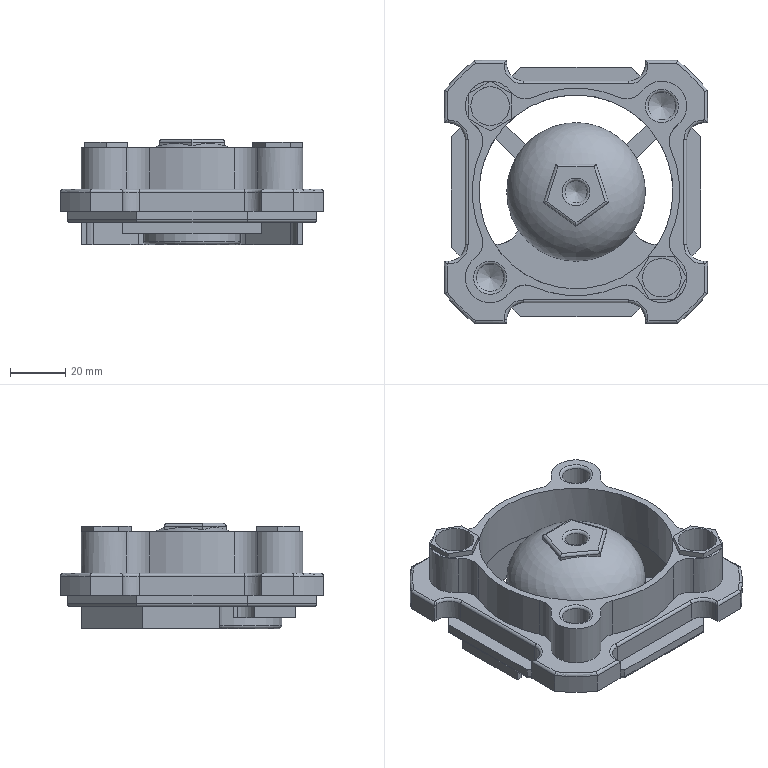NC program | NX | posted with a generic post | part box 95 x 95 x 38 mm
Lines 1358 to 2302 of 59038:
(PLANAR_MILL , TOOL : D20)
N2702 M6
N2704 G54
N2706 G17 G0 G90 X-51.14 Y-59.625 S3000 M3
N2708 G43 Z10. H0
N2710 Z-3.589
N2712 G94 G1 Z-3.789 F2500.
N2714 X-44.435 Y-52.92
N2716 G3 X-44.435 Y-44.435 R6.
N2718 G2 X-44.218 Y-17.351 R19.
N2720 X-44.218 Y17.351 R47.5
N2722 X-17.351 Y44.218 R-19.
N2724 X17.351 Y44.218 R47.5
N2726 X44.218 Y17.351 R-19.
N2728 X44.218 Y-17.351 R47.5
N2730 X17.351 Y-44.218 R-19.
N2732 X-17.351 Y-44.218 R47.5
N2734 X-44.435 Y-44.435 R19.
N2736 G3 X-52.92 Y-44.435 R6.
N2738 G1 X-59.625 Y-51.14
N2740 Z-3.589
N2742 G0 X-51.14 Y-59.625 Z-4.379
N2744 G1 Z-4.579
N2746 X-44.435 Y-52.92
N2748 G3 X-44.435 Y-44.435 R6.
N2750 G2 X-44.218 Y-17.351 R19.
N2752 X-44.218 Y17.351 R47.5
N2754 X-17.351 Y44.218 R-19.
N2756 X17.351 Y44.218 R47.5
N2758 X44.218 Y17.351 R-19.
N2760 X44.218 Y-17.351 R47.5
N2762 X17.351 Y-44.218 R-19.
N2764 X-17.351 Y-44.218 R47.5
N2766 X-44.435 Y-44.435 R19.
N2768 G3 X-52.92 Y-44.435 R6.
N2770 G1 X-59.625 Y-51.14
N2772 Z-4.379
N2774 G0 X-51.14 Y-59.625 Z-5.168
N2776 G1 Z-5.368
N2778 X-44.435 Y-52.92
N2780 G3 X-44.435 Y-44.435 R6.
N2782 G2 X-44.218 Y-17.351 R19.
N2784 X-44.218 Y17.351 R47.5
N2786 X-17.351 Y44.218 R-19.
N2788 X17.351 Y44.218 R47.5
N2790 X44.218 Y17.351 R-19.
N2792 X44.218 Y-17.351 R47.5
N2794 X17.351 Y-44.218 R-19.
N2796 X-17.351 Y-44.218 R47.5
N2798 X-44.435 Y-44.435 R19.
N2800 G3 X-52.92 Y-44.435 R6.
N2802 G1 X-59.625 Y-51.14
N2804 Z-5.168
N2806 G0 X-51.14 Y-59.625 Z-5.958
N2808 G1 Z-6.158
N2810 X-44.435 Y-52.92
N2812 G3 X-44.435 Y-44.435 R6.
N2814 G2 X-44.218 Y-17.351 R19.
N2816 X-44.218 Y17.351 R47.5
N2818 X-17.351 Y44.218 R-19.
N2820 X17.351 Y44.218 R47.5
N2822 X44.218 Y17.351 R-19.
N2824 X44.218 Y-17.351 R47.5
N2826 X17.351 Y-44.218 R-19.
N2828 X-17.351 Y-44.218 R47.5
N2830 X-44.435 Y-44.435 R19.
N2832 G3 X-52.92 Y-44.435 R6.
N2834 G1 X-59.625 Y-51.14
N2836 Z-5.958
N2838 G0 X-51.14 Y-59.625 Z-6.747
N2840 G1 Z-6.947
N2842 X-44.435 Y-52.92
N2844 G3 X-44.435 Y-44.435 R6.
N2846 G2 X-44.218 Y-17.351 R19.
N2848 X-44.218 Y17.351 R47.5
N2850 X-17.351 Y44.218 R-19.
N2852 X17.351 Y44.218 R47.5
N2854 X44.218 Y17.351 R-19.
N2856 X44.218 Y-17.351 R47.5
N2858 X17.351 Y-44.218 R-19.
N2860 X-17.351 Y-44.218 R47.5
N2862 X-44.435 Y-44.435 R19.
N2864 G3 X-52.92 Y-44.435 R6.
N2866 G1 X-59.625 Y-51.14
N2868 Z-6.747
N2870 G0 X-51.14 Y-59.625 Z-7.537
N2872 G1 Z-7.737
N2874 X-44.435 Y-52.92
N2876 G3 X-44.435 Y-44.435 R6.
N2878 G2 X-44.218 Y-17.351 R19.
N2880 X-44.218 Y17.351 R47.5
N2882 X-17.351 Y44.218 R-19.
N2884 X17.351 Y44.218 R47.5
N2886 X44.218 Y17.351 R-19.
N2888 X44.218 Y-17.351 R47.5
N2890 X17.351 Y-44.218 R-19.
N2892 X-17.351 Y-44.218 R47.5
N2894 X-44.435 Y-44.435 R19.
N2896 G3 X-52.92 Y-44.435 R6.
N2898 G1 X-59.625 Y-51.14
N2900 Z-7.537
N2902 G0 X-51.14 Y-59.625 Z-8.326
N2904 G1 Z-8.526
N2906 X-44.435 Y-52.92
N2908 G3 X-44.435 Y-44.435 R6.
N2910 G2 X-44.218 Y-17.351 R19.
N2912 X-44.218 Y17.351 R47.5
N2914 X-17.351 Y44.218 R-19.
N2916 X17.351 Y44.218 R47.5
N2918 X44.218 Y17.351 R-19.
N2920 X44.218 Y-17.351 R47.5
N2922 X17.351 Y-44.218 R-19.
N2924 X-17.351 Y-44.218 R47.5
N2926 X-44.435 Y-44.435 R19.
N2928 G3 X-52.92 Y-44.435 R6.
N2930 G1 X-59.625 Y-51.14
N2932 Z-8.326
N2934 G0 X-51.14 Y-59.625 Z-9.116
N2936 G1 Z-9.316
N2938 X-44.435 Y-52.92
N2940 G3 X-44.435 Y-44.435 R6.
N2942 G2 X-44.218 Y-17.351 R19.
N2944 X-44.218 Y17.351 R47.5
N2946 X-17.351 Y44.218 R-19.
N2948 X17.351 Y44.218 R47.5
N2950 X44.218 Y17.351 R-19.
N2952 X44.218 Y-17.351 R47.5
N2954 X17.351 Y-44.218 R-19.
N2956 X-17.351 Y-44.218 R47.5
N2958 X-44.435 Y-44.435 R19.
N2960 G3 X-52.92 Y-44.435 R6.
N2962 G1 X-59.625 Y-51.14
N2964 Z-9.116
N2966 G0 X-51.14 Y-59.625 Z-9.905
N2968 G1 Z-10.105
N2970 X-44.435 Y-52.92
N2972 G3 X-44.435 Y-44.435 R6.
N2974 G2 X-44.218 Y-17.351 R19.
N2976 X-44.218 Y17.351 R47.5
N2978 X-17.351 Y44.218 R-19.
N2980 X17.351 Y44.218 R47.5
N2982 X44.218 Y17.351 R-19.
N2984 X44.218 Y-17.351 R47.5
N2986 X17.351 Y-44.218 R-19.
N2988 X-17.351 Y-44.218 R47.5
N2990 X-44.435 Y-44.435 R19.
N2992 G3 X-52.92 Y-44.435 R6.
N2994 G1 X-59.625 Y-51.14
N2996 Z-9.905
N2998 G0 X-51.14 Y-59.625 Z-10.695
N3000 G1 Z-10.895
N3002 X-44.435 Y-52.92
N3004 G3 X-44.435 Y-44.435 R6.
N3006 G2 X-44.218 Y-17.351 R19.
N3008 X-44.218 Y17.351 R47.5
N3010 X-17.351 Y44.218 R-19.
N3012 X17.351 Y44.218 R47.5
N3014 X44.218 Y17.351 R-19.
N3016 X44.218 Y-17.351 R47.5
N3018 X17.351 Y-44.218 R-19.
N3020 X-17.351 Y-44.218 R47.5
N3022 X-44.435 Y-44.435 R19.
N3024 G3 X-52.92 Y-44.435 R6.
N3026 G1 X-59.625 Y-51.14
N3028 Z-10.695
N3030 G0 X-51.14 Y-59.625 Z-11.484
N3032 G1 Z-11.684
N3034 X-44.435 Y-52.92
N3036 G3 X-44.435 Y-44.435 R6.
N3038 G2 X-44.218 Y-17.351 R19.
N3040 X-44.218 Y17.351 R47.5
N3042 X-17.351 Y44.218 R-19.
N3044 X17.351 Y44.218 R47.5
N3046 X44.218 Y17.351 R-19.
N3048 X44.218 Y-17.351 R47.5
N3050 X17.351 Y-44.218 R-19.
N3052 X-17.351 Y-44.218 R47.5
N3054 X-44.435 Y-44.435 R19.
N3056 G3 X-52.92 Y-44.435 R6.
N3058 G1 X-59.625 Y-51.14
N3060 Z-11.484
N3062 G0 X-51.14 Y-59.625 Z-12.274
N3064 G1 Z-12.474
N3066 X-44.435 Y-52.92
N3068 G3 X-44.435 Y-44.435 R6.
N3070 G2 X-44.218 Y-17.351 R19.
N3072 X-44.218 Y17.351 R47.5
N3074 X-17.351 Y44.218 R-19.
N3076 X17.351 Y44.218 R47.5
N3078 X44.218 Y17.351 R-19.
N3080 X44.218 Y-17.351 R47.5
N3082 X17.351 Y-44.218 R-19.
N3084 X-17.351 Y-44.218 R47.5
N3086 X-44.435 Y-44.435 R19.
N3088 G3 X-52.92 Y-44.435 R6.
N3090 G1 X-59.625 Y-51.14
N3092 Z-12.274
N3094 G0 X-51.14 Y-59.625 Z-13.063
N3096 G1 Z-13.263
N3098 X-44.435 Y-52.92
N3100 G3 X-44.435 Y-44.435 R6.
N3102 G2 X-44.218 Y-17.351 R19.
N3104 X-44.218 Y17.351 R47.5
N3106 X-17.351 Y44.218 R-19.
N3108 X17.351 Y44.218 R47.5
N3110 X44.218 Y17.351 R-19.
N3112 X44.218 Y-17.351 R47.5
N3114 X17.351 Y-44.218 R-19.
N3116 X-17.351 Y-44.218 R47.5
N3118 X-44.435 Y-44.435 R19.
N3120 G3 X-52.92 Y-44.435 R6.
N3122 G1 X-59.625 Y-51.14
N3124 Z-13.063
N3126 G0 X-51.14 Y-59.625 Z-13.853
N3128 G1 Z-14.053
N3130 X-44.435 Y-52.92
N3132 G3 X-44.435 Y-44.435 R6.
N3134 G2 X-44.218 Y-17.351 R19.
N3136 X-44.218 Y17.351 R47.5
N3138 X-17.351 Y44.218 R-19.
N3140 X17.351 Y44.218 R47.5
N3142 X44.218 Y17.351 R-19.
N3144 X44.218 Y-17.351 R47.5
N3146 X17.351 Y-44.218 R-19.
N3148 X-17.351 Y-44.218 R47.5
N3150 X-44.435 Y-44.435 R19.
N3152 G3 X-52.92 Y-44.435 R6.
N3154 G1 X-59.625 Y-51.14
N3156 Z-13.853
N3158 G0 X-51.14 Y-59.625 Z-14.642
N3160 G1 Z-14.842
N3162 X-44.435 Y-52.92
N3164 G3 X-44.435 Y-44.435 R6.
N3166 G2 X-44.218 Y-17.351 R19.
N3168 X-44.218 Y17.351 R47.5
N3170 X-17.351 Y44.218 R-19.
N3172 X17.351 Y44.218 R47.5
N3174 X44.218 Y17.351 R-19.
N3176 X44.218 Y-17.351 R47.5
N3178 X17.351 Y-44.218 R-19.
N3180 X-17.351 Y-44.218 R47.5
N3182 X-44.435 Y-44.435 R19.
N3184 G3 X-52.92 Y-44.435 R6.
N3186 G1 X-59.625 Y-51.14
N3188 Z-14.642
N3190 G0 X-51.14 Y-59.625 Z-15.432
N3192 G1 Z-15.632
N3194 X-44.435 Y-52.92
N3196 G3 X-44.435 Y-44.435 R6.
N3198 G2 X-44.218 Y-17.351 R19.
N3200 X-44.218 Y17.351 R47.5
N3202 X-17.351 Y44.218 R-19.
N3204 X17.351 Y44.218 R47.5
N3206 X44.218 Y17.351 R-19.
N3208 X44.218 Y-17.351 R47.5
N3210 X17.351 Y-44.218 R-19.
N3212 X-17.351 Y-44.218 R47.5
N3214 X-44.435 Y-44.435 R19.
N3216 G3 X-52.92 Y-44.435 R6.
N3218 G1 X-59.625 Y-51.14
N3220 Z-15.432
N3222 G0 X-51.14 Y-59.625 Z-16.221
N3224 G1 Z-16.421
N3226 X-44.435 Y-52.92
N3228 G3 X-44.435 Y-44.435 R6.
N3230 G2 X-44.218 Y-17.351 R19.
N3232 X-44.218 Y17.351 R47.5
N3234 X-17.351 Y44.218 R-19.
N3236 X17.351 Y44.218 R47.5
N3238 X44.218 Y17.351 R-19.
N3240 X44.218 Y-17.351 R47.5
N3242 X17.351 Y-44.218 R-19.
N3244 X-17.351 Y-44.218 R47.5
N3246 X-44.435 Y-44.435 R19.
N3248 G3 X-52.92 Y-44.435 R6.
N3250 G1 X-59.625 Y-51.14
N3252 Z-16.221
N3254 G0 X-51.14 Y-59.625 Z-17.011
N3256 G1 Z-17.211
N3258 X-44.435 Y-52.92
N3260 G3 X-44.435 Y-44.435 R6.
N3262 G2 X-44.218 Y-17.351 R19.
N3264 X-44.218 Y17.351 R47.5
N3266 X-17.351 Y44.218 R-19.
N3268 X17.351 Y44.218 R47.5
N3270 X44.218 Y17.351 R-19.
N3272 X44.218 Y-17.351 R47.5
N3274 X17.351 Y-44.218 R-19.
N3276 X-17.351 Y-44.218 R47.5
N3278 X-44.435 Y-44.435 R19.
N3280 G3 X-52.92 Y-44.435 R6.
N3282 G1 X-59.625 Y-51.14
N3284 Z-17.011
N3286 G0 X-51.14 Y-59.625 Z-17.8
N3288 G1 Z-18.
N3290 X-44.435 Y-52.92
N3292 G3 X-44.435 Y-44.435 R6.
N3294 G2 X-44.218 Y-17.351 R19.
N3296 X-44.218 Y17.351 R47.5
N3298 X-17.351 Y44.218 R-19.
N3300 X17.351 Y44.218 R47.5
N3302 X44.218 Y17.351 R-19.
N3304 X44.218 Y-17.351 R47.5
N3306 X17.351 Y-44.218 R-19.
N3308 X-17.351 Y-44.218 R47.5
N3310 X-44.435 Y-44.435 R19.
N3312 G3 X-52.92 Y-44.435 R6.
N3314 G1 X-59.625 Y-51.14
N3316 Z-17.8
N3318 G0 Z10.
(PLANAR_MILL_COPY , TOOL : D20)
N3320 X-66. Y-6.
N3322 Z-18.6
N3324 G1 Z-18.8
N3326 X-56.
N3328 G3 X-50. Y0. R6.
N3330 G1 Y15.318
N3332 G2 X-57.5 Y25. R10.
N3334 G1 Y36.657
N3336 G2 X-55.417 Y42.767 R10.
N3338 X-42.767 Y55.417 R70.
N3340 X-36.657 Y57.5 R10.
N3342 G1 X-25.
N3344 G2 X-15.318 Y50. R10.
N3346 G1 X15.318
N3348 G2 X25. Y57.5 R10.
N3350 G1 X36.657
N3352 G2 X42.767 Y55.417 R10.
N3354 X55.417 Y42.767 R70.
N3356 X57.5 Y36.657 R10.
N3358 G1 Y25.
N3360 G2 X50. Y15.318 R10.
N3362 G1 Y-15.318
N3364 G2 X57.5 Y-25. R10.
N3366 G1 Y-36.657
N3368 G2 X55.417 Y-42.767 R10.
N3370 X42.767 Y-55.417 R70.
N3372 X36.657 Y-57.5 R10.
N3374 G1 X25.
N3376 G2 X15.318 Y-50. R10.
N3378 G1 X-15.318
N3380 G2 X-25. Y-57.5 R10.
N3382 G1 X-36.657
N3384 G2 X-42.767 Y-55.417 R10.
N3386 X-55.417 Y-42.767 R70.
N3388 X-57.5 Y-36.657 R10.
N3390 G1 Y-25.
N3392 G2 X-50. Y-15.318 R10.
N3394 G1 Y0.
N3396 G3 X-56. Y6. R6.
N3398 G1 X-66.
N3400 Z-18.6
N3402 G0 Y-6. Z-19.4
N3404 G1 Z-19.6
N3406 X-56.
N3408 G3 X-50. Y0. R6.
N3410 G1 Y15.318
N3412 G2 X-57.5 Y25. R10.
N3414 G1 Y36.657
N3416 G2 X-55.417 Y42.767 R10.
N3418 X-42.767 Y55.417 R70.
N3420 X-36.657 Y57.5 R10.
N3422 G1 X-25.
N3424 G2 X-15.318 Y50. R10.
N3426 G1 X15.318
N3428 G2 X25. Y57.5 R10.
N3430 G1 X36.657
N3432 G2 X42.767 Y55.417 R10.
N3434 X55.417 Y42.767 R70.
N3436 X57.5 Y36.657 R10.
N3438 G1 Y25.
N3440 G2 X50. Y15.318 R10.
N3442 G1 Y-15.318
N3444 G2 X57.5 Y-25. R10.
N3446 G1 Y-36.657
N3448 G2 X55.417 Y-42.767 R10.
N3450 X42.767 Y-55.417 R70.
N3452 X36.657 Y-57.5 R10.
N3454 G1 X25.
N3456 G2 X15.318 Y-50. R10.
N3458 G1 X-15.318
N3460 G2 X-25. Y-57.5 R10.
N3462 G1 X-36.657
N3464 G2 X-42.767 Y-55.417 R10.
N3466 X-55.417 Y-42.767 R70.
N3468 X-57.5 Y-36.657 R10.
N3470 G1 Y-25.
N3472 G2 X-50. Y-15.318 R10.
N3474 G1 Y0.
N3476 G3 X-56. Y6. R6.
N3478 G1 X-66.
N3480 Z-19.4
N3482 G0 Y-6. Z-20.2
N3484 G1 Z-20.4
N3486 X-56.
N3488 G3 X-50. Y0. R6.
N3490 G1 Y15.318
N3492 G2 X-57.5 Y25. R10.
N3494 G1 Y36.657
N3496 G2 X-55.417 Y42.767 R10.
N3498 X-42.767 Y55.417 R70.
N3500 X-36.657 Y57.5 R10.
N3502 G1 X-25.
N3504 G2 X-15.318 Y50. R10.
N3506 G1 X15.318
N3508 G2 X25. Y57.5 R10.
N3510 G1 X36.657
N3512 G2 X42.767 Y55.417 R10.
N3514 X55.417 Y42.767 R70.
N3516 X57.5 Y36.657 R10.
N3518 G1 Y25.
N3520 G2 X50. Y15.318 R10.
N3522 G1 Y-15.318
N3524 G2 X57.5 Y-25. R10.
N3526 G1 Y-36.657
N3528 G2 X55.417 Y-42.767 R10.
N3530 X42.767 Y-55.417 R70.
N3532 X36.657 Y-57.5 R10.
N3534 G1 X25.
N3536 G2 X15.318 Y-50. R10.
N3538 G1 X-15.318
N3540 G2 X-25. Y-57.5 R10.
N3542 G1 X-36.657
N3544 G2 X-42.767 Y-55.417 R10.
N3546 X-55.417 Y-42.767 R70.
N3548 X-57.5 Y-36.657 R10.
N3550 G1 Y-25.
N3552 G2 X-50. Y-15.318 R10.
N3554 G1 Y0.
N3556 G3 X-56. Y6. R6.
N3558 G1 X-66.
N3560 Z-20.2
N3562 G0 Y-6. Z-21.
N3564 G1 Z-21.2
N3566 X-56.
N3568 G3 X-50. Y0. R6.
N3570 G1 Y15.318
N3572 G2 X-57.5 Y25. R10.
N3574 G1 Y36.657
N3576 G2 X-55.417 Y42.767 R10.
N3578 X-42.767 Y55.417 R70.
N3580 X-36.657 Y57.5 R10.
N3582 G1 X-25.
N3584 G2 X-15.318 Y50. R10.
N3586 G1 X15.318
N3588 G2 X25. Y57.5 R10.
N3590 G1 X36.657
N3592 G2 X42.767 Y55.417 R10.
N3594 X55.417 Y42.767 R70.
N3596 X57.5 Y36.657 R10.
N3598 G1 Y25.
N3600 G2 X50. Y15.318 R10.
N3602 G1 Y-15.318
N3604 G2 X57.5 Y-25. R10.
N3606 G1 Y-36.657
N3608 G2 X55.417 Y-42.767 R10.
N3610 X42.767 Y-55.417 R70.
N3612 X36.657 Y-57.5 R10.
N3614 G1 X25.
N3616 G2 X15.318 Y-50. R10.
N3618 G1 X-15.318
N3620 G2 X-25. Y-57.5 R10.
N3622 G1 X-36.657
N3624 G2 X-42.767 Y-55.417 R10.
N3626 X-55.417 Y-42.767 R70.
N3628 X-57.5 Y-36.657 R10.
N3630 G1 Y-25.
N3632 G2 X-50. Y-15.318 R10.
N3634 G1 Y0.
N3636 G3 X-56. Y6. R6.
N3638 G1 X-66.
N3640 Z-21.
N3642 G0 Y-6. Z-21.8
N3644 G1 Z-22.
N3646 X-56.
N3648 G3 X-50. Y0. R6.
N3650 G1 Y15.318
N3652 G2 X-57.5 Y25. R10.
N3654 G1 Y36.657
N3656 G2 X-55.417 Y42.767 R10.
N3658 X-42.767 Y55.417 R70.
N3660 X-36.657 Y57.5 R10.
N3662 G1 X-25.
N3664 G2 X-15.318 Y50. R10.
N3666 G1 X15.318
N3668 G2 X25. Y57.5 R10.
N3670 G1 X36.657
N3672 G2 X42.767 Y55.417 R10.
N3674 X55.417 Y42.767 R70.
N3676 X57.5 Y36.657 R10.
N3678 G1 Y25.
N3680 G2 X50. Y15.318 R10.
N3682 G1 Y-15.318
N3684 G2 X57.5 Y-25. R10.
N3686 G1 Y-36.657
N3688 G2 X55.417 Y-42.767 R10.
N3690 X42.767 Y-55.417 R70.
N3692 X36.657 Y-57.5 R10.
N3694 G1 X25.
N3696 G2 X15.318 Y-50. R10.
N3698 G1 X-15.318
N3700 G2 X-25. Y-57.5 R10.
N3702 G1 X-36.657
N3704 G2 X-42.767 Y-55.417 R10.
N3706 X-55.417 Y-42.767 R70.
N3708 X-57.5 Y-36.657 R10.
N3710 G1 Y-25.
N3712 G2 X-50. Y-15.318 R10.
N3714 G1 Y0.
N3716 G3 X-56. Y6. R6.
N3718 G1 X-66.
N3720 Z-21.8
N3722 G0 Y-6. Z-22.6
N3724 G1 Z-22.8
N3726 X-56.
N3728 G3 X-50. Y0. R6.
N3730 G1 Y15.318
N3732 G2 X-57.5 Y25. R10.
N3734 G1 Y36.657
N3736 G2 X-55.417 Y42.767 R10.
N3738 X-42.767 Y55.417 R70.
N3740 X-36.657 Y57.5 R10.
N3742 G1 X-25.
N3744 G2 X-15.318 Y50. R10.
N3746 G1 X15.318
N3748 G2 X25. Y57.5 R10.
N3750 G1 X36.657
N3752 G2 X42.767 Y55.417 R10.
N3754 X55.417 Y42.767 R70.
N3756 X57.5 Y36.657 R10.
N3758 G1 Y25.
N3760 G2 X50. Y15.318 R10.
N3762 G1 Y-15.318
N3764 G2 X57.5 Y-25. R10.
N3766 G1 Y-36.657
N3768 G2 X55.417 Y-42.767 R10.
N3770 X42.767 Y-55.417 R70.
N3772 X36.657 Y-57.5 R10.
N3774 G1 X25.
N3776 G2 X15.318 Y-50. R10.
N3778 G1 X-15.318
N3780 G2 X-25. Y-57.5 R10.
N3782 G1 X-36.657
N3784 G2 X-42.767 Y-55.417 R10.
N3786 X-55.417 Y-42.767 R70.
N3788 X-57.5 Y-36.657 R10.
N3790 G1 Y-25.
N3792 G2 X-50. Y-15.318 R10.
N3794 G1 Y0.
N3796 G3 X-56. Y6. R6.
N3798 G1 X-66.
N3800 Z-22.6
N3802 G0 Y-6. Z-23.4
N3804 G1 Z-23.6
N3806 X-56.
N3808 G3 X-50. Y0. R6.
N3810 G1 Y15.318
N3812 G2 X-57.5 Y25. R10.
N3814 G1 Y36.657
N3816 G2 X-55.417 Y42.767 R10.
N3818 X-42.767 Y55.417 R70.
N3820 X-36.657 Y57.5 R10.
N3822 G1 X-25.
N3824 G2 X-15.318 Y50. R10.
N3826 G1 X15.318
N3828 G2 X25. Y57.5 R10.
N3830 G1 X36.657
N3832 G2 X42.767 Y55.417 R10.
N3834 X55.417 Y42.767 R70.
N3836 X57.5 Y36.657 R10.
N3838 G1 Y25.
N3840 G2 X50. Y15.318 R10.
N3842 G1 Y-15.318
N3844 G2 X57.5 Y-25. R10.
N3846 G1 Y-36.657
N3848 G2 X55.417 Y-42.767 R10.
N3850 X42.767 Y-55.417 R70.
N3852 X36.657 Y-57.5 R10.
N3854 G1 X25.
N3856 G2 X15.318 Y-50. R10.
N3858 G1 X-15.318
N3860 G2 X-25. Y-57.5 R10.
N3862 G1 X-36.657
N3864 G2 X-42.767 Y-55.417 R10.
N3866 X-55.417 Y-42.767 R70.
N3868 X-57.5 Y-36.657 R10.
N3870 G1 Y-25.
N3872 G2 X-50. Y-15.318 R10.
N3874 G1 Y0.
N3876 G3 X-56. Y6. R6.
N3878 G1 X-66.
N3880 Z-23.4
N3882 G0 Y-6. Z-24.2
N3884 G1 Z-24.4
N3886 X-56.
N3888 G3 X-50. Y0. R6.
N3890 G1 Y15.318
N3892 G2 X-57.5 Y25. R10.
N3894 G1 Y36.657
N3896 G2 X-55.417 Y42.767 R10.
N3898 X-42.767 Y55.417 R70.
N3900 X-36.657 Y57.5 R10.
N3902 G1 X-25.
N3904 G2 X-15.318 Y50. R10.
N3906 G1 X15.318
N3908 G2 X25. Y57.5 R10.
N3910 G1 X36.657
N3912 G2 X42.767 Y55.417 R10.
N3914 X55.417 Y42.767 R70.
N3916 X57.5 Y36.657 R10.
N3918 G1 Y25.
N3920 G2 X50. Y15.318 R10.
N3922 G1 Y-15.318
N3924 G2 X57.5 Y-25. R10.
N3926 G1 Y-36.657
N3928 G2 X55.417 Y-42.767 R10.
N3930 X42.767 Y-55.417 R70.
N3932 X36.657 Y-57.5 R10.
N3934 G1 X25.
N3936 G2 X15.318 Y-50. R10.
N3938 G1 X-15.318
N3940 G2 X-25. Y-57.5 R10.
N3942 G1 X-36.657
N3944 G2 X-42.767 Y-55.417 R10.
N3946 X-55.417 Y-42.767 R70.
N3948 X-57.5 Y-36.657 R10.
N3950 G1 Y-25.
N3952 G2 X-50. Y-15.318 R10.
N3954 G1 Y0.
N3956 G3 X-56. Y6. R6.
N3958 G1 X-66.
N3960 Z-24.2
N3962 G0 Y-6. Z-25.
N3964 G1 Z-25.2
N3966 X-56.
N3968 G3 X-50. Y0. R6.
N3970 G1 Y15.318
N3972 G2 X-57.5 Y25. R10.
N3974 G1 Y36.657
N3976 G2 X-55.417 Y42.767 R10.
N3978 X-42.767 Y55.417 R70.
N3980 X-36.657 Y57.5 R10.
N3982 G1 X-25.
N3984 G2 X-15.318 Y50. R10.
N3986 G1 X15.318
N3988 G2 X25. Y57.5 R10.
N3990 G1 X36.657
N3992 G2 X42.767 Y55.417 R10.
N3994 X55.417 Y42.767 R70.
N3996 X57.5 Y36.657 R10.
N3998 G1 Y25.
N4000 G2 X50. Y15.318 R10.
N4002 G1 Y-15.318
N4004 G2 X57.5 Y-25. R10.
N4006 G1 Y-36.657
N4008 G2 X55.417 Y-42.767 R10.
N4010 X42.767 Y-55.417 R70.
N4012 X36.657 Y-57.5 R10.
N4014 G1 X25.
N4016 G2 X15.318 Y-50. R10.
N4018 G1 X-15.318
N4020 G2 X-25. Y-57.5 R10.
N4022 G1 X-36.657
N4024 G2 X-42.767 Y-55.417 R10.
N4026 X-55.417 Y-42.767 R70.
N4028 X-57.5 Y-36.657 R10.
N4030 G1 Y-25.
N4032 G2 X-50. Y-15.318 R10.
N4034 G1 Y0.
N4036 G3 X-56. Y6. R6.
N4038 G1 X-66.
N4040 Z-25.
N4042 G0 Y-6. Z-25.8
N4044 G1 Z-26.
N4046 X-56.
N4048 G3 X-50. Y0. R6.
N4050 G1 Y15.318
N4052 G2 X-57.5 Y25. R10.
N4054 G1 Y36.657
N4056 G2 X-55.417 Y42.767 R10.
N4058 X-42.767 Y55.417 R70.
N4060 X-36.657 Y57.5 R10.
N4062 G1 X-25.
N4064 G2 X-15.318 Y50. R10.
N4066 G1 X15.318
N4068 G2 X25. Y57.5 R10.
N4070 G1 X36.657
N4072 G2 X42.767 Y55.417 R10.
N4074 X55.417 Y42.767 R70.
N4076 X57.5 Y36.657 R10.
N4078 G1 Y25.
N4080 G2 X50. Y15.318 R10.
N4082 G1 Y-15.318
N4084 G2 X57.5 Y-25. R10.
N4086 G1 Y-36.657
N4088 G2 X55.417 Y-42.767 R10.
N4090 X42.767 Y-55.417 R70.
N4092 X36.657 Y-57.5 R10.
N4094 G1 X25.
N4096 G2 X15.318 Y-50. R10.
N4098 G1 X-15.318
N4100 G2 X-25. Y-57.5 R10.
N4102 G1 X-36.657
N4104 G2 X-42.767 Y-55.417 R10.
N4106 X-55.417 Y-42.767 R70.
N4108 X-57.5 Y-36.657 R10.
N4110 G1 Y-25.
N4112 G2 X-50. Y-15.318 R10.
N4114 G1 Y0.
N4116 G3 X-56. Y6. R6.
N4118 G1 X-66.
N4120 Z-25.8
N4122 G0 Z10.
N4124 M5
(SPOT_DRILLING , TOOL : 点钻)
N4126 M6
N4128 G54
N4130 G17 G0 G90 X31. Y31. S0 M3
N4132 G43 Z10. H0
N4134 G94 G82 G99 Z-1. F250. P200 R2.
N4136 Y-31.
N4138 X0. Y0.
N4140 X-31. Y31.
N4142 Y-31.
N4144 G80
N4146 G0 X-31. Y-31. Z10.
N4148 M5
(DRILLING , TOOL : D10)
N4150 M6
N4152 G54
N4154 G17 G0 G90 X31. Y-31. S0 M3
N4156 G43 Z10. H0
N4158 G94 G81 G99 Z-18. F250. R2.
N4160 Y31. Z-18.004 R0.
N4162 G80
N4164 G0 Z3.
N4166 G81 X0. Y0. Z-1. F250. R3.
N4168 X-31. Y31. Z-18. R2.
N4170 Y-31. Z-18.004 R0.
N4172 G80
N4174 G0 X-31. Y-31. Z10.
N4176 M5
(HOLE_MILLING , TOOL : D8)
N4178 M6
N4180 G54
N4182 G17 G0 G90 X31. Y-31. S3000 M3
N4184 G43 Z10. H0
N4186 Z-1.
N4188 G94 G3 X32.5 Y-32.5 R1.5 F2500.
N4190 X34. Y-31. R1.5
N4192 X34. Y-31. Z-1.2 I-3. J0.
N4194 X34. Y-31. Z-1.4 I-3. J0.
N4196 X34. Y-31. Z-1.6 I-3. J0.
N4198 X34. Y-31. Z-1.8 I-3. J0.
N4200 X34. Y-31. Z-2. I-3. J0.
N4202 X34. Y-31. Z-2.2 I-3. J0.
N4204 X34. Y-31. Z-2.4 I-3. J0.
N4206 X34. Y-31. Z-2.6 I-3. J0.
N4208 X34. Y-31. Z-2.8 I-3. J0.
N4210 X34. Y-31. Z-3. I-3. J0.
N4212 X34. Y-31. Z-3.2 I-3. J0.
N4214 X34. Y-31. Z-3.4 I-3. J0.
N4216 X34. Y-31. Z-3.6 I-3. J0.
N4218 X34. Y-31. Z-3.8 I-3. J0.
N4220 X34. Y-31. Z-4. I-3. J0.
N4222 X34. Y-31. Z-4.2 I-3. J0.
N4224 X34. Y-31. Z-4.4 I-3. J0.
N4226 X34. Y-31. Z-4.6 I-3. J0.
N4228 X34. Y-31. Z-4.8 I-3. J0.
N4230 X34. Y-31. Z-5. I-3. J0.
N4232 X34. Y-31. Z-5.2 I-3. J0.
N4234 X34. Y-31. Z-5.4 I-3. J0.
N4236 X34. Y-31. Z-5.6 I-3. J0.
N4238 X34. Y-31. Z-5.8 I-3. J0.
N4240 X34. Y-31. Z-6. I-3. J0.
N4242 X34. Y-31. Z-6.2 I-3. J0.
N4244 X34. Y-31. Z-6.4 I-3. J0.
N4246 X34. Y-31. Z-6.6 I-3. J0.
N4248 X34. Y-31. Z-6.8 I-3. J0.
N4250 X34. Y-31. Z-7. I-3. J0.
N4252 X34. Y-31. Z-7.2 I-3. J0.
N4254 X34. Y-31. Z-7.4 I-3. J0.
N4256 X34. Y-31. Z-7.6 I-3. J0.
N4258 X34. Y-31. Z-7.8 I-3. J0.
N4260 X34. Y-31. Z-8. I-3. J0.
N4262 X34. Y-31. Z-8.2 I-3. J0.
N4264 X34. Y-31. Z-8.4 I-3. J0.
N4266 X34. Y-31. Z-8.6 I-3. J0.
N4268 X34. Y-31. Z-8.8 I-3. J0.
N4270 X34. Y-31. Z-9. I-3. J0.
N4272 X34. Y-31. Z-9.2 I-3. J0.
N4274 X34. Y-31. Z-9.4 I-3. J0.
N4276 X34. Y-31. Z-9.6 I-3. J0.
N4278 X34. Y-31. Z-9.8 I-3. J0.
N4280 X34. Y-31. Z-10. I-3. J0.
N4282 X34. Y-31. Z-10.2 I-3. J0.
N4284 X34. Y-31. Z-10.4 I-3. J0.
N4286 X34. Y-31. Z-10.6 I-3. J0.
N4288 X34. Y-31. Z-10.8 I-3. J0.
N4290 X34. Y-31. Z-11. I-3. J0.
N4292 X34. Y-31. Z-11.2 I-3. J0.
N4294 X34. Y-31. Z-11.4 I-3. J0.
N4296 X34. Y-31. Z-11.6 I-3. J0.
N4298 X34. Y-31. Z-11.8 I-3. J0.
N4300 X34. Y-31. Z-12. I-3. J0.
N4302 X34. Y-31. Z-12.2 I-3. J0.
N4304 X34. Y-31. Z-12.4 I-3. J0.
N4306 X34. Y-31. Z-12.6 I-3. J0.
N4308 X34. Y-31. Z-12.8 I-3. J0.
N4310 X34. Y-31. Z-13. I-3. J0.
N4312 X34. Y-31. Z-13.2 I-3. J0.
N4314 X34. Y-31. Z-13.4 I-3. J0.
N4316 X34. Y-31. Z-13.6 I-3. J0.
N4318 X34. Y-31. Z-13.8 I-3. J0.
N4320 X34. Y-31. Z-14. I-3. J0.
N4322 X34. Y-31. Z-14.2 I-3. J0.
N4324 X34. Y-31. Z-14.4 I-3. J0.
N4326 X34. Y-31. Z-14.6 I-3. J0.
N4328 X34. Y-31. Z-14.8 I-3. J0.
N4330 X34. Y-31. Z-15. I-3. J0.
N4332 X34. Y-31. Z-15.2 I-3. J0.
N4334 X34. Y-31. Z-15.4 I-3. J0.
N4336 X34. Y-31. Z-15.6 I-3. J0.
N4338 X34. Y-31. Z-15.8 I-3. J0.
N4340 X34. Y-31. Z-16. I-3. J0.
N4342 X34. Y-31. Z-16.2 I-3. J0.
N4344 X34. Y-31. Z-16.4 I-3. J0.
N4346 X34. Y-31. Z-16.6 I-3. J0.
N4348 X34. Y-31. Z-16.8 I-3. J0.
N4350 X34. Y-31. Z-17. I-3. J0.
N4352 X34. Y-31. Z-17.2 I-3. J0.
N4354 X34. Y-31. Z-17.4 I-3. J0.
N4356 X34. Y-31. Z-17.6 I-3. J0.
N4358 X34. Y-31. Z-17.8 I-3. J0.
N4360 X34. Y-31. Z-18. I-3. J0.
N4362 X31. Y-28. R3.
N4364 X34. Y-31. R-3.
N4366 X32.5 Y-29.5 R1.5
N4368 X31. Y-31. R1.5
N4370 G0 Z10.
N4372 X-31. Y31.
N4374 Z-1.
N4376 G3 X-29.5 Y29.5 R1.5
N4378 X-28. Y31. R1.5
N4380 X-28. Y31. Z-1.2 I-3. J0.
N4382 X-28. Y31. Z-1.4 I-3. J0.
N4384 X-28. Y31. Z-1.6 I-3. J0.
N4386 X-28. Y31. Z-1.8 I-3. J0.
N4388 X-28. Y31. Z-2. I-3. J0.
N4390 X-28. Y31. Z-2.2 I-3. J0.
N4392 X-28. Y31. Z-2.4 I-3. J0.
N4394 X-28. Y31. Z-2.6 I-3. J0.
N4396 X-28. Y31. Z-2.8 I-3. J0.
N4398 X-28. Y31. Z-3. I-3. J0.
N4400 X-28. Y31. Z-3.2 I-3. J0.
N4402 X-28. Y31. Z-3.4 I-3. J0.
N4404 X-28. Y31. Z-3.6 I-3. J0.
N4406 X-28. Y31. Z-3.8 I-3. J0.
N4408 X-28. Y31. Z-4. I-3. J0.
N4410 X-28. Y31. Z-4.2 I-3. J0.
N4412 X-28. Y31. Z-4.4 I-3. J0.
N4414 X-28. Y31. Z-4.6 I-3. J0.
N4416 X-28. Y31. Z-4.8 I-3. J0.
N4418 X-28. Y31. Z-5. I-3. J0.
N4420 X-28. Y31. Z-5.2 I-3. J0.
N4422 X-28. Y31. Z-5.4 I-3. J0.
N4424 X-28. Y31. Z-5.6 I-3. J0.
N4426 X-28. Y31. Z-5.8 I-3. J0.
N4428 X-28. Y31. Z-6. I-3. J0.
N4430 X-28. Y31. Z-6.2 I-3. J0.
N4432 X-28. Y31. Z-6.4 I-3. J0.
N4434 X-28. Y31. Z-6.6 I-3. J0.
N4436 X-28. Y31. Z-6.8 I-3. J0.
N4438 X-28. Y31. Z-7. I-3. J0.
N4440 X-28. Y31. Z-7.2 I-3. J0.
N4442 X-28. Y31. Z-7.4 I-3. J0.
N4444 X-28. Y31. Z-7.6 I-3. J0.
N4446 X-28. Y31. Z-7.8 I-3. J0.
N4448 X-28. Y31. Z-8. I-3. J0.
N4450 X-28. Y31. Z-8.2 I-3. J0.
N4452 X-28. Y31. Z-8.4 I-3. J0.
N4454 X-28. Y31. Z-8.6 I-3. J0.
N4456 X-28. Y31. Z-8.8 I-3. J0.
N4458 X-28. Y31. Z-9. I-3. J0.
N4460 X-28. Y31. Z-9.2 I-3. J0.
N4462 X-28. Y31. Z-9.4 I-3. J0.
N4464 X-28. Y31. Z-9.6 I-3. J0.
N4466 X-28. Y31. Z-9.8 I-3. J0.
N4468 X-28. Y31. Z-10. I-3. J0.
N4470 X-28. Y31. Z-10.2 I-3. J0.
N4472 X-28. Y31. Z-10.4 I-3. J0.
N4474 X-28. Y31. Z-10.6 I-3. J0.
N4476 X-28. Y31. Z-10.8 I-3. J0.
N4478 X-28. Y31. Z-11. I-3. J0.
N4480 X-28. Y31. Z-11.2 I-3. J0.
N4482 X-28. Y31. Z-11.4 I-3. J0.
N4484 X-28. Y31. Z-11.6 I-3. J0.
N4486 X-28. Y31. Z-11.8 I-3. J0.
N4488 X-28. Y31. Z-12. I-3. J0.
N4490 X-28. Y31. Z-12.2 I-3. J0.
N4492 X-28. Y31. Z-12.4 I-3. J0.
N4494 X-28. Y31. Z-12.6 I-3. J0.
N4496 X-28. Y31. Z-12.8 I-3. J0.
N4498 X-28. Y31. Z-13. I-3. J0.
N4500 X-28. Y31. Z-13.2 I-3. J0.
N4502 X-28. Y31. Z-13.4 I-3. J0.
N4504 X-28. Y31. Z-13.6 I-3. J0.
N4506 X-28. Y31. Z-13.8 I-3. J0.
N4508 X-28. Y31. Z-14. I-3. J0.
N4510 X-28. Y31. Z-14.2 I-3. J0.
N4512 X-28. Y31. Z-14.4 I-3. J0.
N4514 X-28. Y31. Z-14.6 I-3. J0.
N4516 X-28. Y31. Z-14.8 I-3. J0.
N4518 X-28. Y31. Z-15. I-3. J0.
N4520 X-28. Y31. Z-15.2 I-3. J0.
N4522 X-28. Y31. Z-15.4 I-3. J0.
N4524 X-28. Y31. Z-15.6 I-3. J0.
N4526 X-28. Y31. Z-15.8 I-3. J0.
N4528 X-28. Y31. Z-16. I-3. J0.
N4530 X-28. Y31. Z-16.2 I-3. J0.
N4532 X-28. Y31. Z-16.4 I-3. J0.
N4534 X-28. Y31. Z-16.6 I-3. J0.
N4536 X-28. Y31. Z-16.8 I-3. J0.
N4538 X-28. Y31. Z-17. I-3. J0.
N4540 X-28. Y31. Z-17.2 I-3. J0.
N4542 X-28. Y31. Z-17.4 I-3. J0.
N4544 X-28. Y31. Z-17.6 I-3. J0.
N4546 X-28. Y31. Z-17.8 I-3. J0.
N4548 X-28. Y31. Z-18. I-3. J0.
N4550 X-31. Y34. R3.
N4552 X-28. Y31. R-3.
N4554 X-29.5 Y32.5 R1.5
N4556 X-31. Y31. R1.5
N4558 G0 Z10.
N4560 M5